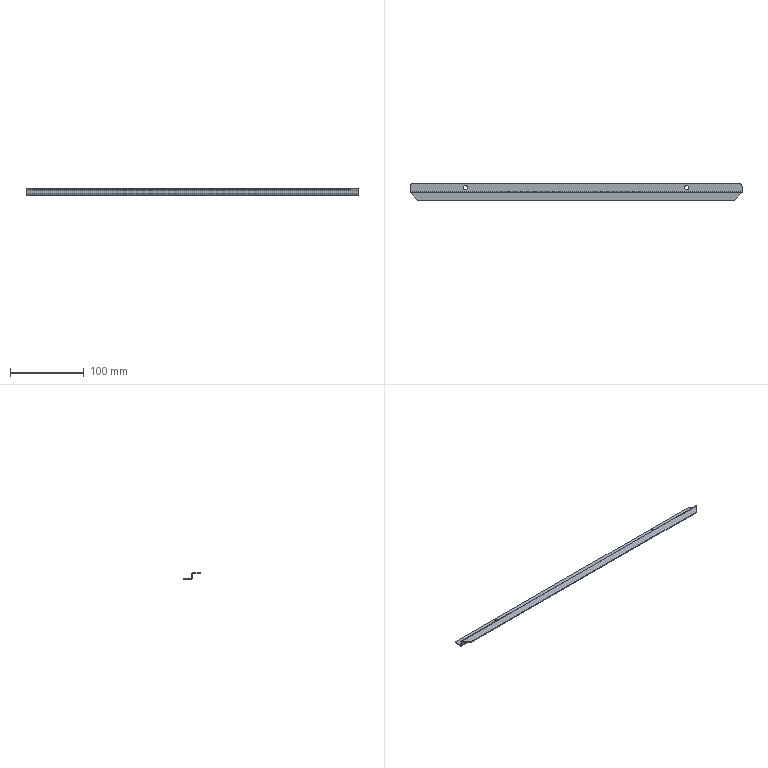Part | SolidWorks | features Chamfer 1, Fillet 1, FlatPattern 1, HoleWzd 1, SMBaseFlange 1, SheetMetal 1 | 1 solid | 28 faces | box 450 x 22 x 8.2 mm | volume 15097 mm3 | plane 18 | cylinder 10 | commonest cylinder face diameters 6 x6 0.4 x2 2.8 x2
STEP:
#1=CARTESIAN_POINT('',(-153.,7.,0.));
#2=VERTEX_POINT('',#1);
#3=CARTESIAN_POINT('',(-147.,7.,0.));
#4=VERTEX_POINT('',#3);
#5=CARTESIAN_POINT('',(-150.,7.,0.));
#6=DIRECTION('',(0.,0.,1.));
#7=DIRECTION('',(1.,0.,0.));
#8=AXIS2_PLACEMENT_3D('',#5,#6,#7);
#9=CIRCLE('',#8,3.);
#10=EDGE_CURVE('',#2,#4,#9,.T.);
#11=ORIENTED_EDGE('',*,*,#10,.F.);
#12=CARTESIAN_POINT('',(-153.,7.,1.2));
#13=VERTEX_POINT('',#12);
#14=CARTESIAN_POINT('',(-153.,7.,1.2));
#15=DIRECTION('',(0.,0.,1.));
#16=VECTOR('',#15,1000.);
#17=LINE('',#14,#16);
#18=EDGE_CURVE('',#2,#13,#17,.T.);
#19=ORIENTED_EDGE('',*,*,#18,.T.);
#20=CARTESIAN_POINT('',(-147.,7.,1.2));
#21=VERTEX_POINT('',#20);
#22=CARTESIAN_POINT('',(-150.,7.,1.2));
#23=DIRECTION('',(0.,0.,1.));
#24=DIRECTION('',(1.,0.,0.));
#25=AXIS2_PLACEMENT_3D('',#22,#23,#24);
#26=CIRCLE('',#25,3.);
#27=EDGE_CURVE('',#13,#21,#26,.T.);
#28=ORIENTED_EDGE('',*,*,#27,.T.);
#29=CARTESIAN_POINT('',(-147.,7.,1.2));
#30=DIRECTION('',(0.,0.,1.));
#31=VECTOR('',#30,1000.);
#32=LINE('',#29,#31);
#33=EDGE_CURVE('',#4,#21,#32,.T.);
#34=ORIENTED_EDGE('',*,*,#33,.F.);
#35=EDGE_LOOP('',(#11,#19,#28,#34));
#36=FACE_OUTER_BOUND('',#35,.T.);
#37=CARTESIAN_POINT('',(-150.,7.,1.2));
#38=DIRECTION('',(0.,0.,1.));
#39=DIRECTION('',(1.,0.,0.));
#40=AXIS2_PLACEMENT_3D('',#37,#38,#39);
#41=CYLINDRICAL_SURFACE('',#40,3.);
#42=ADVANCED_FACE('',(#36),#41,.F.);
#43=CARTESIAN_POINT('',(147.,7.,0.));
#44=VERTEX_POINT('',#43);
#45=CARTESIAN_POINT('',(153.,7.,0.));
#46=VERTEX_POINT('',#45);
#47=CARTESIAN_POINT('',(150.,7.,0.));
#48=DIRECTION('',(0.,0.,1.));
#49=DIRECTION('',(1.,0.,0.));
#50=AXIS2_PLACEMENT_3D('',#47,#48,#49);
#51=CIRCLE('',#50,3.);
#52=EDGE_CURVE('',#44,#46,#51,.T.);
#53=ORIENTED_EDGE('',*,*,#52,.F.);
#54=CARTESIAN_POINT('',(147.,7.,1.2));
#55=VERTEX_POINT('',#54);
#56=CARTESIAN_POINT('',(147.,7.,1.2));
#57=DIRECTION('',(0.,0.,1.));
#58=VECTOR('',#57,1000.);
#59=LINE('',#56,#58);
#60=EDGE_CURVE('',#44,#55,#59,.T.);
#61=ORIENTED_EDGE('',*,*,#60,.T.);
#62=CARTESIAN_POINT('',(153.,7.,1.2));
#63=VERTEX_POINT('',#62);
#64=CARTESIAN_POINT('',(150.,7.,1.2));
#65=DIRECTION('',(0.,0.,1.));
#66=DIRECTION('',(1.,0.,0.));
#67=AXIS2_PLACEMENT_3D('',#64,#65,#66);
#68=CIRCLE('',#67,3.);
#69=EDGE_CURVE('',#55,#63,#68,.T.);
#70=ORIENTED_EDGE('',*,*,#69,.T.);
#71=CARTESIAN_POINT('',(153.,7.,1.2));
#72=DIRECTION('',(0.,0.,1.));
#73=VECTOR('',#72,1000.);
#74=LINE('',#71,#73);
#75=EDGE_CURVE('',#46,#63,#74,.T.);
#76=ORIENTED_EDGE('',*,*,#75,.F.);
#77=EDGE_LOOP('',(#53,#61,#70,#76));
#78=FACE_OUTER_BOUND('',#77,.T.);
#79=CARTESIAN_POINT('',(150.,7.,1.2));
#80=DIRECTION('',(0.,0.,1.));
#81=DIRECTION('',(1.,0.,0.));
#82=AXIS2_PLACEMENT_3D('',#79,#80,#81);
#83=CYLINDRICAL_SURFACE('',#82,3.);
#84=ADVANCED_FACE('',(#78),#83,.F.);
#85=CARTESIAN_POINT('',(225.,0.,8.186));
#86=VERTEX_POINT('',#85);
#87=CARTESIAN_POINT('',(225.,1.2,6.8));
#88=VERTEX_POINT('',#87);
#89=CARTESIAN_POINT('',(225.,-0.2,6.8));
#90=DIRECTION('',(-1.,0.,0.));
#91=DIRECTION('',(0.,0.,-1.));
#92=AXIS2_PLACEMENT_3D('',#89,#90,#91);
#93=CIRCLE('',#92,1.4);
#94=EDGE_CURVE('',#86,#88,#93,.T.);
#95=ORIENTED_EDGE('',*,*,#94,.F.);
#96=CARTESIAN_POINT('',(225.,0.,6.8));
#97=VERTEX_POINT('',#96);
#98=CARTESIAN_POINT('',(225.,0.,7.));
#99=DIRECTION('',(0.,0.,-1.));
#100=VECTOR('',#99,1000.);
#101=LINE('',#98,#100);
#102=EDGE_CURVE('',#86,#97,#101,.T.);
#103=ORIENTED_EDGE('',*,*,#102,.T.);
#104=CARTESIAN_POINT('',(225.,1.2,6.8));
#105=DIRECTION('',(0.,-1.,0.));
#106=VECTOR('',#105,1000.);
#107=LINE('',#104,#106);
#108=EDGE_CURVE('',#88,#97,#107,.T.);
#109=ORIENTED_EDGE('',*,*,#108,.F.);
#110=EDGE_LOOP('',(#95,#103,#109));
#111=FACE_OUTER_BOUND('',#110,.T.);
#112=CARTESIAN_POINT('',(225.,-0.2,7.));
#113=DIRECTION('',(1.,0.,0.));
#114=DIRECTION('',(0.,0.,-1.));
#115=AXIS2_PLACEMENT_3D('',#112,#113,#114);
#116=PLANE('',#115);
#117=ADVANCED_FACE('',(#111),#116,.T.);
#118=CARTESIAN_POINT('',(-225.,0.,6.8));
#119=VERTEX_POINT('',#118);
#120=CARTESIAN_POINT('',(-225.,1.2,6.8));
#121=VERTEX_POINT('',#120);
#122=CARTESIAN_POINT('',(-225.,0.,6.8));
#123=DIRECTION('',(0.,1.,0.));
#124=VECTOR('',#123,1000.);
#125=LINE('',#122,#124);
#126=EDGE_CURVE('',#119,#121,#125,.T.);
#127=ORIENTED_EDGE('',*,*,#126,.F.);
#128=CARTESIAN_POINT('',(-225.,0.,8.186));
#129=VERTEX_POINT('',#128);
#130=CARTESIAN_POINT('',(-225.,0.,6.8));
#131=DIRECTION('',(0.,0.,1.));
#132=VECTOR('',#131,1000.);
#133=LINE('',#130,#132);
#134=EDGE_CURVE('',#119,#129,#133,.T.);
#135=ORIENTED_EDGE('',*,*,#134,.T.);
#136=CARTESIAN_POINT('',(-225.,-0.2,6.8));
#137=DIRECTION('',(-1.,0.,0.));
#138=DIRECTION('',(0.,0.,-1.));
#139=AXIS2_PLACEMENT_3D('',#136,#137,#138);
#140=CIRCLE('',#139,1.4);
#141=EDGE_CURVE('',#129,#121,#140,.T.);
#142=ORIENTED_EDGE('',*,*,#141,.T.);
#143=EDGE_LOOP('',(#127,#135,#142));
#144=FACE_OUTER_BOUND('',#143,.T.);
#145=CARTESIAN_POINT('',(-225.,0.,6.8));
#146=DIRECTION('',(-1.,0.,0.));
#147=DIRECTION('',(0.,0.,1.));
#148=AXIS2_PLACEMENT_3D('',#145,#146,#147);
#149=PLANE('',#148);
#150=ADVANCED_FACE('',(#144),#149,.T.);
#151=CARTESIAN_POINT('',(-225.,0.,1.4));
#152=VERTEX_POINT('',#151);
#153=CARTESIAN_POINT('',(-225.,0.,0.));
#154=DIRECTION('',(0.,0.,-1.));
#155=VECTOR('',#154,1000.);
#156=LINE('',#153,#155);
#157=EDGE_CURVE('',#119,#152,#156,.T.);
#158=ORIENTED_EDGE('',*,*,#157,.F.);
#159=ORIENTED_EDGE('',*,*,#126,.T.);
#160=CARTESIAN_POINT('',(-225.,1.2,1.4));
#161=VERTEX_POINT('',#160);
#162=CARTESIAN_POINT('',(-225.,1.2,0.));
#163=DIRECTION('',(0.,0.,-1.));
#164=VECTOR('',#163,1000.);
#165=LINE('',#162,#164);
#166=EDGE_CURVE('',#121,#161,#165,.T.);
#167=ORIENTED_EDGE('',*,*,#166,.T.);
#168=CARTESIAN_POINT('',(-225.,1.2,1.4));
#169=DIRECTION('',(0.,-1.,0.));
#170=VECTOR('',#169,1000.);
#171=LINE('',#168,#170);
#172=EDGE_CURVE('',#161,#152,#171,.T.);
#173=ORIENTED_EDGE('',*,*,#172,.T.);
#174=EDGE_LOOP('',(#158,#159,#167,#173));
#175=FACE_OUTER_BOUND('',#174,.T.);
#176=CARTESIAN_POINT('',(-225.,-0.2,8.2));
#177=DIRECTION('',(-1.,0.,0.));
#178=DIRECTION('',(0.,0.,1.));
#179=AXIS2_PLACEMENT_3D('',#176,#177,#178);
#180=PLANE('',#179);
#181=ADVANCED_FACE('',(#175),#180,.T.);
#182=CARTESIAN_POINT('',(225.,0.,1.4));
#183=VERTEX_POINT('',#182);
#184=CARTESIAN_POINT('',(225.,1.2,1.4));
#185=VERTEX_POINT('',#184);
#186=CARTESIAN_POINT('',(225.,0.,1.4));
#187=DIRECTION('',(0.,1.,0.));
#188=VECTOR('',#187,1000.);
#189=LINE('',#186,#188);
#190=EDGE_CURVE('',#183,#185,#189,.T.);
#191=ORIENTED_EDGE('',*,*,#190,.F.);
#192=CARTESIAN_POINT('',(225.,1.4,0.));
#193=VERTEX_POINT('',#192);
#194=CARTESIAN_POINT('',(225.,1.4,1.4));
#195=DIRECTION('',(1.,0.,0.));
#196=DIRECTION('',(0.,0.,1.));
#197=AXIS2_PLACEMENT_3D('',#194,#195,#196);
#198=CIRCLE('',#197,1.4);
#199=EDGE_CURVE('',#183,#193,#198,.T.);
#200=ORIENTED_EDGE('',*,*,#199,.T.);
#201=CARTESIAN_POINT('',(225.,1.4,1.2));
#202=VERTEX_POINT('',#201);
#203=CARTESIAN_POINT('',(225.,1.4,1.2));
#204=DIRECTION('',(0.,0.,-1.));
#205=VECTOR('',#204,1000.);
#206=LINE('',#203,#205);
#207=EDGE_CURVE('',#202,#193,#206,.T.);
#208=ORIENTED_EDGE('',*,*,#207,.F.);
#209=CARTESIAN_POINT('',(225.,1.4,1.4));
#210=DIRECTION('',(1.,0.,0.));
#211=DIRECTION('',(0.,0.,-1.));
#212=AXIS2_PLACEMENT_3D('',#209,#210,#211);
#213=CIRCLE('',#212,0.2);
#214=EDGE_CURVE('',#185,#202,#213,.T.);
#215=ORIENTED_EDGE('',*,*,#214,.F.);
#216=EDGE_LOOP('',(#191,#200,#208,#215));
#217=FACE_OUTER_BOUND('',#216,.T.);
#218=CARTESIAN_POINT('',(225.,0.,1.4));
#219=DIRECTION('',(1.,0.,0.));
#220=DIRECTION('',(0.,0.,-1.));
#221=AXIS2_PLACEMENT_3D('',#218,#219,#220);
#222=PLANE('',#221);
#223=ADVANCED_FACE('',(#217),#222,.T.);
#224=CARTESIAN_POINT('',(225.,0.,0.));
#225=DIRECTION('',(0.,0.,-1.));
#226=VECTOR('',#225,1000.);
#227=LINE('',#224,#226);
#228=EDGE_CURVE('',#97,#183,#227,.T.);
#229=ORIENTED_EDGE('',*,*,#228,.T.);
#230=ORIENTED_EDGE('',*,*,#190,.T.);
#231=CARTESIAN_POINT('',(225.,1.2,0.));
#232=DIRECTION('',(0.,0.,-1.));
#233=VECTOR('',#232,1000.);
#234=LINE('',#231,#233);
#235=EDGE_CURVE('',#88,#185,#234,.T.);
#236=ORIENTED_EDGE('',*,*,#235,.F.);
#237=ORIENTED_EDGE('',*,*,#108,.T.);
#238=EDGE_LOOP('',(#229,#230,#236,#237));
#239=FACE_OUTER_BOUND('',#238,.T.);
#240=CARTESIAN_POINT('',(225.,1.4,1.2));
#241=DIRECTION('',(1.,0.,0.));
#242=DIRECTION('',(0.,0.,-1.));
#243=AXIS2_PLACEMENT_3D('',#240,#241,#242);
#244=PLANE('',#243);
#245=ADVANCED_FACE('',(#239),#244,.T.);
#246=CARTESIAN_POINT('',(-225.,1.4,0.));
#247=VERTEX_POINT('',#246);
#248=CARTESIAN_POINT('',(-225.,1.4,1.2));
#249=VERTEX_POINT('',#248);
#250=CARTESIAN_POINT('',(-225.,1.4,0.));
#251=DIRECTION('',(0.,0.,1.));
#252=VECTOR('',#251,1000.);
#253=LINE('',#250,#252);
#254=EDGE_CURVE('',#247,#249,#253,.T.);
#255=ORIENTED_EDGE('',*,*,#254,.F.);
#256=CARTESIAN_POINT('',(-225.,1.4,1.4));
#257=DIRECTION('',(1.,0.,0.));
#258=DIRECTION('',(0.,0.,1.));
#259=AXIS2_PLACEMENT_3D('',#256,#257,#258);
#260=CIRCLE('',#259,1.4);
#261=EDGE_CURVE('',#152,#247,#260,.T.);
#262=ORIENTED_EDGE('',*,*,#261,.F.);
#263=ORIENTED_EDGE('',*,*,#172,.F.);
#264=CARTESIAN_POINT('',(-225.,1.4,1.4));
#265=DIRECTION('',(1.,0.,0.));
#266=DIRECTION('',(0.,0.,-1.));
#267=AXIS2_PLACEMENT_3D('',#264,#265,#266);
#268=CIRCLE('',#267,0.2);
#269=EDGE_CURVE('',#161,#249,#268,.T.);
#270=ORIENTED_EDGE('',*,*,#269,.T.);
#271=EDGE_LOOP('',(#255,#262,#263,#270));
#272=FACE_OUTER_BOUND('',#271,.T.);
#273=CARTESIAN_POINT('',(-225.,1.4,0.));
#274=DIRECTION('',(-1.,0.,0.));
#275=DIRECTION('',(0.,0.,1.));
#276=AXIS2_PLACEMENT_3D('',#273,#274,#275);
#277=PLANE('',#276);
#278=ADVANCED_FACE('',(#272),#277,.T.);
#279=CARTESIAN_POINT('',(-225.,9.,1.2));
#280=VERTEX_POINT('',#279);
#281=CARTESIAN_POINT('',(-225.,0.,1.2));
#282=DIRECTION('',(0.,1.,0.));
#283=VECTOR('',#282,1000.);
#284=LINE('',#281,#283);
#285=EDGE_CURVE('',#249,#280,#284,.T.);
#286=ORIENTED_EDGE('',*,*,#285,.T.);
#287=CARTESIAN_POINT('',(-225.,9.,0.));
#288=VERTEX_POINT('',#287);
#289=CARTESIAN_POINT('',(-225.,9.,1.4));
#290=DIRECTION('',(0.,0.,-1.));
#291=VECTOR('',#290,1000.);
#292=LINE('',#289,#291);
#293=EDGE_CURVE('',#280,#288,#292,.T.);
#294=ORIENTED_EDGE('',*,*,#293,.T.);
#295=CARTESIAN_POINT('',(-225.,0.,0.));
#296=DIRECTION('',(0.,1.,0.));
#297=VECTOR('',#296,1000.);
#298=LINE('',#295,#297);
#299=EDGE_CURVE('',#247,#288,#298,.T.);
#300=ORIENTED_EDGE('',*,*,#299,.F.);
#301=ORIENTED_EDGE('',*,*,#254,.T.);
#302=EDGE_LOOP('',(#286,#294,#300,#301));
#303=FACE_OUTER_BOUND('',#302,.T.);
#304=CARTESIAN_POINT('',(-225.,1.2,1.4));
#305=DIRECTION('',(-1.,0.,0.));
#306=DIRECTION('',(0.,0.,1.));
#307=AXIS2_PLACEMENT_3D('',#304,#305,#306);
#308=PLANE('',#307);
#309=ADVANCED_FACE('',(#303),#308,.T.);
#310=CARTESIAN_POINT('',(-150.,7.,0.));
#311=DIRECTION('',(0.,0.,1.));
#312=DIRECTION('',(1.,0.,0.));
#313=AXIS2_PLACEMENT_3D('',#310,#311,#312);
#314=CIRCLE('',#313,3.);
#315=EDGE_CURVE('',#4,#2,#314,.T.);
#316=ORIENTED_EDGE('',*,*,#315,.T.);
#317=ORIENTED_EDGE('',*,*,#10,.T.);
#318=EDGE_LOOP('',(#316,#317));
#319=FACE_BOUND('',#318,.T.);
#320=CARTESIAN_POINT('',(150.,7.,0.));
#321=DIRECTION('',(0.,0.,1.));
#322=DIRECTION('',(1.,0.,0.));
#323=AXIS2_PLACEMENT_3D('',#320,#321,#322);
#324=CIRCLE('',#323,3.);
#325=EDGE_CURVE('',#46,#44,#324,.T.);
#326=ORIENTED_EDGE('',*,*,#325,.T.);
#327=ORIENTED_EDGE('',*,*,#52,.T.);
#328=EDGE_LOOP('',(#326,#327));
#329=FACE_BOUND('',#328,.T.);
#330=ORIENTED_EDGE('',*,*,#299,.T.);
#331=CARTESIAN_POINT('',(-222.,12.,0.));
#332=VERTEX_POINT('',#331);
#333=CARTESIAN_POINT('',(-222.,9.,0.));
#334=DIRECTION('',(0.,0.,-1.));
#335=DIRECTION('',(1.,0.,0.));
#336=AXIS2_PLACEMENT_3D('',#333,#334,#335);
#337=CIRCLE('',#336,3.);
#338=EDGE_CURVE('',#288,#332,#337,.T.);
#339=ORIENTED_EDGE('',*,*,#338,.T.);
#340=CARTESIAN_POINT('',(222.,12.,0.));
#341=VERTEX_POINT('',#340);
#342=CARTESIAN_POINT('',(225.,12.,0.));
#343=DIRECTION('',(-1.,0.,0.));
#344=VECTOR('',#343,1000.);
#345=LINE('',#342,#344);
#346=EDGE_CURVE('',#341,#332,#345,.T.);
#347=ORIENTED_EDGE('',*,*,#346,.F.);
#348=CARTESIAN_POINT('',(225.,9.,0.));
#349=VERTEX_POINT('',#348);
#350=CARTESIAN_POINT('',(222.,9.,0.));
#351=DIRECTION('',(0.,0.,-1.));
#352=DIRECTION('',(1.,0.,0.));
#353=AXIS2_PLACEMENT_3D('',#350,#351,#352);
#354=CIRCLE('',#353,3.);
#355=EDGE_CURVE('',#341,#349,#354,.T.);
#356=ORIENTED_EDGE('',*,*,#355,.T.);
#357=CARTESIAN_POINT('',(225.,0.,0.));
#358=DIRECTION('',(0.,1.,0.));
#359=VECTOR('',#358,1000.);
#360=LINE('',#357,#359);
#361=EDGE_CURVE('',#193,#349,#360,.T.);
#362=ORIENTED_EDGE('',*,*,#361,.F.);
#363=CARTESIAN_POINT('',(225.,1.4,0.));
#364=DIRECTION('',(-1.,0.,0.));
#365=VECTOR('',#364,1000.);
#366=LINE('',#363,#365);
#367=EDGE_CURVE('',#193,#247,#366,.T.);
#368=ORIENTED_EDGE('',*,*,#367,.T.);
#369=EDGE_LOOP('',(#330,#339,#347,#356,#362,#368));
#370=FACE_OUTER_BOUND('',#369,.T.);
#371=CARTESIAN_POINT('',(225.,0.,0.));
#372=DIRECTION('',(0.,0.,1.));
#373=DIRECTION('',(1.,0.,0.));
#374=AXIS2_PLACEMENT_3D('',#371,#372,#373);
#375=PLANE('',#374);
#376=ADVANCED_FACE('',(#319,#329,#370),#375,.F.);
#377=ORIENTED_EDGE('',*,*,#346,.T.);
#378=CARTESIAN_POINT('',(-222.,12.,1.2));
#379=VERTEX_POINT('',#378);
#380=CARTESIAN_POINT('',(-222.,12.,1.2));
#381=DIRECTION('',(0.,0.,1.));
#382=VECTOR('',#381,1000.);
#383=LINE('',#380,#382);
#384=EDGE_CURVE('',#332,#379,#383,.T.);
#385=ORIENTED_EDGE('',*,*,#384,.T.);
#386=CARTESIAN_POINT('',(222.,12.,1.2));
#387=VERTEX_POINT('',#386);
#388=CARTESIAN_POINT('',(225.,12.,1.2));
#389=DIRECTION('',(-1.,0.,0.));
#390=VECTOR('',#389,1000.);
#391=LINE('',#388,#390);
#392=EDGE_CURVE('',#387,#379,#391,.T.);
#393=ORIENTED_EDGE('',*,*,#392,.F.);
#394=CARTESIAN_POINT('',(222.,12.,1.2));
#395=DIRECTION('',(0.,0.,-1.));
#396=VECTOR('',#395,1000.);
#397=LINE('',#394,#396);
#398=EDGE_CURVE('',#387,#341,#397,.T.);
#399=ORIENTED_EDGE('',*,*,#398,.T.);
#400=EDGE_LOOP('',(#377,#385,#393,#399));
#401=FACE_OUTER_BOUND('',#400,.T.);
#402=CARTESIAN_POINT('',(225.,12.,1.2));
#403=DIRECTION('',(0.,1.,0.));
#404=DIRECTION('',(0.,0.,1.));
#405=AXIS2_PLACEMENT_3D('',#402,#403,#404);
#406=PLANE('',#405);
#407=ADVANCED_FACE('',(#401),#406,.T.);
#408=CARTESIAN_POINT('',(-150.,7.,1.2));
#409=DIRECTION('',(0.,0.,1.));
#410=DIRECTION('',(1.,0.,0.));
#411=AXIS2_PLACEMENT_3D('',#408,#409,#410);
#412=CIRCLE('',#411,3.);
#413=EDGE_CURVE('',#21,#13,#412,.T.);
#414=ORIENTED_EDGE('',*,*,#413,.F.);
#415=ORIENTED_EDGE('',*,*,#27,.F.);
#416=EDGE_LOOP('',(#414,#415));
#417=FACE_BOUND('',#416,.T.);
#418=CARTESIAN_POINT('',(150.,7.,1.2));
#419=DIRECTION('',(0.,0.,1.));
#420=DIRECTION('',(1.,0.,0.));
#421=AXIS2_PLACEMENT_3D('',#418,#419,#420);
#422=CIRCLE('',#421,3.);
#423=EDGE_CURVE('',#63,#55,#422,.T.);
#424=ORIENTED_EDGE('',*,*,#423,.F.);
#425=ORIENTED_EDGE('',*,*,#69,.F.);
#426=EDGE_LOOP('',(#424,#425));
#427=FACE_BOUND('',#426,.T.);
#428=ORIENTED_EDGE('',*,*,#392,.T.);
#429=CARTESIAN_POINT('',(-222.,9.,1.2));
#430=DIRECTION('',(0.,0.,1.));
#431=DIRECTION('',(1.,0.,0.));
#432=AXIS2_PLACEMENT_3D('',#429,#430,#431);
#433=CIRCLE('',#432,3.);
#434=EDGE_CURVE('',#379,#280,#433,.T.);
#435=ORIENTED_EDGE('',*,*,#434,.T.);
#436=ORIENTED_EDGE('',*,*,#285,.F.);
#437=CARTESIAN_POINT('',(225.,1.4,1.2));
#438=DIRECTION('',(-1.,0.,0.));
#439=VECTOR('',#438,1000.);
#440=LINE('',#437,#439);
#441=EDGE_CURVE('',#202,#249,#440,.T.);
#442=ORIENTED_EDGE('',*,*,#441,.F.);
#443=CARTESIAN_POINT('',(225.,9.,1.2));
#444=VERTEX_POINT('',#443);
#445=CARTESIAN_POINT('',(225.,0.,1.2));
#446=DIRECTION('',(0.,1.,0.));
#447=VECTOR('',#446,1000.);
#448=LINE('',#445,#447);
#449=EDGE_CURVE('',#202,#444,#448,.T.);
#450=ORIENTED_EDGE('',*,*,#449,.T.);
#451=CARTESIAN_POINT('',(222.,9.,1.2));
#452=DIRECTION('',(0.,0.,1.));
#453=DIRECTION('',(1.,0.,0.));
#454=AXIS2_PLACEMENT_3D('',#451,#452,#453);
#455=CIRCLE('',#454,3.);
#456=EDGE_CURVE('',#444,#387,#455,.T.);
#457=ORIENTED_EDGE('',*,*,#456,.T.);
#458=EDGE_LOOP('',(#428,#435,#436,#442,#450,#457));
#459=FACE_OUTER_BOUND('',#458,.T.);
#460=CARTESIAN_POINT('',(225.,0.,1.2));
#461=DIRECTION('',(0.,0.,1.));
#462=DIRECTION('',(1.,0.,0.));
#463=AXIS2_PLACEMENT_3D('',#460,#461,#462);
#464=PLANE('',#463);
#465=ADVANCED_FACE('',(#417,#427,#459),#464,.T.);
#466=ORIENTED_EDGE('',*,*,#269,.F.);
#467=CARTESIAN_POINT('',(225.,1.2,1.4));
#468=DIRECTION('',(-1.,0.,0.));
#469=VECTOR('',#468,1000.);
#470=LINE('',#467,#469);
#471=EDGE_CURVE('',#185,#161,#470,.T.);
#472=ORIENTED_EDGE('',*,*,#471,.F.);
#473=ORIENTED_EDGE('',*,*,#214,.T.);
#474=ORIENTED_EDGE('',*,*,#441,.T.);
#475=EDGE_LOOP('',(#466,#472,#473,#474));
#476=FACE_OUTER_BOUND('',#475,.T.);
#477=CARTESIAN_POINT('',(225.,1.4,1.4));
#478=DIRECTION('',(-1.,0.,0.));
#479=DIRECTION('',(0.,0.,1.));
#480=AXIS2_PLACEMENT_3D('',#477,#478,#479);
#481=CYLINDRICAL_SURFACE('',#480,0.2);
#482=ADVANCED_FACE('',(#476),#481,.F.);
#483=ORIENTED_EDGE('',*,*,#166,.F.);
#484=CARTESIAN_POINT('',(225.,1.2,6.8));
#485=DIRECTION('',(-1.,0.,0.));
#486=VECTOR('',#485,1000.);
#487=LINE('',#484,#486);
#488=EDGE_CURVE('',#88,#121,#487,.T.);
#489=ORIENTED_EDGE('',*,*,#488,.F.);
#490=ORIENTED_EDGE('',*,*,#235,.T.);
#491=ORIENTED_EDGE('',*,*,#471,.T.);
#492=EDGE_LOOP('',(#483,#489,#490,#491));
#493=FACE_OUTER_BOUND('',#492,.T.);
#494=CARTESIAN_POINT('',(225.,1.2,0.));
#495=DIRECTION('',(0.,1.,0.));
#496=DIRECTION('',(0.,0.,1.));
#497=AXIS2_PLACEMENT_3D('',#494,#495,#496);
#498=PLANE('',#497);
#499=ADVANCED_FACE('',(#493),#498,.T.);
#500=CARTESIAN_POINT('',(224.8,-0.2,8.2));
#501=VERTEX_POINT('',#500);
#502=CARTESIAN_POINT('',(-224.8,-0.2,8.2));
#503=VERTEX_POINT('',#502);
#504=CARTESIAN_POINT('',(225.,-0.2,8.2));
#505=DIRECTION('',(-1.,0.,0.));
#506=VECTOR('',#505,1000.);
#507=LINE('',#504,#506);
#508=EDGE_CURVE('',#501,#503,#507,.T.);
#509=ORIENTED_EDGE('',*,*,#508,.F.);
#510=CARTESIAN_POINT('',(224.8,-0.2,8.2));
#511=CARTESIAN_POINT('',(224.867,-0.133,8.2));
#512=CARTESIAN_POINT('',(224.934,-0.06627,8.195));
#513=CARTESIAN_POINT('',(225.,0.,8.186));
#514=(BOUNDED_CURVE()B_SPLINE_CURVE(3,(#510,#511,#512,#513),.UNSPECIFIED.,.F.,.T.)B_SPLINE_CURVE_WITH_KNOTS((4,4),(1.571,1.714),.UNSPECIFIED.)CURVE()GEOMETRIC_REPRESENTATION_ITEM()RATIONAL_B_SPLINE_CURVE((1.,0.9983,0.9983,1.))REPRESENTATION_ITEM(''));
#515=EDGE_CURVE('',#501,#86,#514,.T.);
#516=ORIENTED_EDGE('',*,*,#515,.T.);
#517=ORIENTED_EDGE('',*,*,#94,.T.);
#518=ORIENTED_EDGE('',*,*,#488,.T.);
#519=ORIENTED_EDGE('',*,*,#141,.F.);
#520=CARTESIAN_POINT('',(-225.,0.,8.186));
#521=CARTESIAN_POINT('',(-224.934,-0.06627,8.195));
#522=CARTESIAN_POINT('',(-224.867,-0.133,8.2));
#523=CARTESIAN_POINT('',(-224.8,-0.2,8.2));
#524=(BOUNDED_CURVE()B_SPLINE_CURVE(3,(#520,#521,#522,#523),.UNSPECIFIED.,.F.,.T.)B_SPLINE_CURVE_WITH_KNOTS((4,4),(1.427,1.571),.UNSPECIFIED.)CURVE()GEOMETRIC_REPRESENTATION_ITEM()RATIONAL_B_SPLINE_CURVE((1.,0.9983,0.9983,1.))REPRESENTATION_ITEM(''));
#525=EDGE_CURVE('',#129,#503,#524,.T.);
#526=ORIENTED_EDGE('',*,*,#525,.T.);
#527=EDGE_LOOP('',(#509,#516,#517,#518,#519,#526));
#528=FACE_OUTER_BOUND('',#527,.T.);
#529=CARTESIAN_POINT('',(225.,-0.2,6.8));
#530=DIRECTION('',(-1.,0.,0.));
#531=DIRECTION('',(0.,0.,1.));
#532=AXIS2_PLACEMENT_3D('',#529,#530,#531);
#533=CYLINDRICAL_SURFACE('',#532,1.4);
#534=ADVANCED_FACE('',(#528),#533,.T.);
#535=CARTESIAN_POINT('',(215.,-10.,8.2));
#536=VERTEX_POINT('',#535);
#537=CARTESIAN_POINT('',(-215.,-10.,8.2));
#538=VERTEX_POINT('',#537);
#539=CARTESIAN_POINT('',(225.,-10.,8.2));
#540=DIRECTION('',(-1.,0.,0.));
#541=VECTOR('',#540,1000.);
#542=LINE('',#539,#541);
#543=EDGE_CURVE('',#536,#538,#542,.T.);
#544=ORIENTED_EDGE('',*,*,#543,.F.);
#545=CARTESIAN_POINT('',(225.,0.,8.2));
#546=DIRECTION('',(0.7071,0.7071,0.));
#547=VECTOR('',#546,1000.);
#548=LINE('',#545,#547);
#549=EDGE_CURVE('',#536,#501,#548,.T.);
#550=ORIENTED_EDGE('',*,*,#549,.T.);
#551=ORIENTED_EDGE('',*,*,#508,.T.);
#552=CARTESIAN_POINT('',(0.,-225.,8.2));
#553=DIRECTION('',(0.7071,-0.7071,0.));
#554=VECTOR('',#553,1000.);
#555=LINE('',#552,#554);
#556=EDGE_CURVE('',#503,#538,#555,.T.);
#557=ORIENTED_EDGE('',*,*,#556,.T.);
#558=EDGE_LOOP('',(#544,#550,#551,#557));
#559=FACE_OUTER_BOUND('',#558,.T.);
#560=CARTESIAN_POINT('',(225.,0.,8.2));
#561=DIRECTION('',(0.,0.,1.));
#562=DIRECTION('',(0.,-1.,0.));
#563=AXIS2_PLACEMENT_3D('',#560,#561,#562);
#564=PLANE('',#563);
#565=ADVANCED_FACE('',(#559),#564,.T.);
#566=CARTESIAN_POINT('',(215.,-10.,7.));
#567=VERTEX_POINT('',#566);
#568=CARTESIAN_POINT('',(-215.,-10.,7.));
#569=VERTEX_POINT('',#568);
#570=CARTESIAN_POINT('',(225.,-10.,7.));
#571=DIRECTION('',(-1.,0.,0.));
#572=VECTOR('',#571,1000.);
#573=LINE('',#570,#572);
#574=EDGE_CURVE('',#567,#569,#573,.T.);
#575=ORIENTED_EDGE('',*,*,#574,.F.);
#576=CARTESIAN_POINT('',(215.,-10.,7.));
#577=DIRECTION('',(0.,0.,1.));
#578=VECTOR('',#577,1000.);
#579=LINE('',#576,#578);
#580=EDGE_CURVE('',#567,#536,#579,.T.);
#581=ORIENTED_EDGE('',*,*,#580,.T.);
#582=ORIENTED_EDGE('',*,*,#543,.T.);
#583=CARTESIAN_POINT('',(-215.,-10.,7.));
#584=DIRECTION('',(0.,0.,-1.));
#585=VECTOR('',#584,1000.);
#586=LINE('',#583,#585);
#587=EDGE_CURVE('',#538,#569,#586,.T.);
#588=ORIENTED_EDGE('',*,*,#587,.T.);
#589=EDGE_LOOP('',(#575,#581,#582,#588));
#590=FACE_OUTER_BOUND('',#589,.T.);
#591=CARTESIAN_POINT('',(225.,-10.,7.));
#592=DIRECTION('',(0.,-1.,0.));
#593=DIRECTION('',(0.,0.,-1.));
#594=AXIS2_PLACEMENT_3D('',#591,#592,#593);
#595=PLANE('',#594);
#596=ADVANCED_FACE('',(#590),#595,.T.);
#597=CARTESIAN_POINT('',(224.8,-0.2,7.));
#598=VERTEX_POINT('',#597);
#599=CARTESIAN_POINT('',(-224.8,-0.2,7.));
#600=VERTEX_POINT('',#599);
#601=CARTESIAN_POINT('',(225.,-0.2,7.));
#602=DIRECTION('',(-1.,0.,0.));
#603=VECTOR('',#602,1000.);
#604=LINE('',#601,#603);
#605=EDGE_CURVE('',#598,#600,#604,.T.);
#606=ORIENTED_EDGE('',*,*,#605,.F.);
#607=CARTESIAN_POINT('',(215.,-10.,7.));
#608=DIRECTION('',(-0.7071,-0.7071,0.));
#609=VECTOR('',#608,1000.);
#610=LINE('',#607,#609);
#611=EDGE_CURVE('',#598,#567,#610,.T.);
#612=ORIENTED_EDGE('',*,*,#611,.T.);
#613=ORIENTED_EDGE('',*,*,#574,.T.);
#614=CARTESIAN_POINT('',(-225.,0.,7.));
#615=DIRECTION('',(-0.7071,0.7071,0.));
#616=VECTOR('',#615,1000.);
#617=LINE('',#614,#616);
#618=EDGE_CURVE('',#569,#600,#617,.T.);
#619=ORIENTED_EDGE('',*,*,#618,.T.);
#620=EDGE_LOOP('',(#606,#612,#613,#619));
#621=FACE_OUTER_BOUND('',#620,.T.);
#622=CARTESIAN_POINT('',(225.,0.,7.));
#623=DIRECTION('',(0.,0.,1.));
#624=DIRECTION('',(0.,-1.,0.));
#625=AXIS2_PLACEMENT_3D('',#622,#623,#624);
#626=PLANE('',#625);
#627=ADVANCED_FACE('',(#621),#626,.F.);
#628=CARTESIAN_POINT('',(225.,0.,6.8));
#629=DIRECTION('',(-1.,0.,0.));
#630=VECTOR('',#629,1000.);
#631=LINE('',#628,#630);
#632=EDGE_CURVE('',#97,#119,#631,.T.);
#633=ORIENTED_EDGE('',*,*,#632,.F.);
#634=CARTESIAN_POINT('',(225.,0.,6.8));
#635=CARTESIAN_POINT('',(225.,0.,6.917));
#636=CARTESIAN_POINT('',(224.917,-0.08284,7.));
#637=CARTESIAN_POINT('',(224.8,-0.2,7.));
#638=(BOUNDED_CURVE()B_SPLINE_CURVE(3,(#634,#635,#636,#637),.UNSPECIFIED.,.F.,.F.)B_SPLINE_CURVE_WITH_KNOTS((4,4),(3.142,4.712),.UNSPECIFIED.)CURVE()GEOMETRIC_REPRESENTATION_ITEM()RATIONAL_B_SPLINE_CURVE((1.,0.8047,0.8047,1.))REPRESENTATION_ITEM(''));
#639=EDGE_CURVE('',#97,#598,#638,.T.);
#640=ORIENTED_EDGE('',*,*,#639,.T.);
#641=ORIENTED_EDGE('',*,*,#605,.T.);
#642=CARTESIAN_POINT('',(-224.8,-0.2,7.));
#643=CARTESIAN_POINT('',(-224.917,-0.08284,7.));
#644=CARTESIAN_POINT('',(-225.,0.,6.917));
#645=CARTESIAN_POINT('',(-225.,0.,6.8));
#646=(BOUNDED_CURVE()B_SPLINE_CURVE(3,(#642,#643,#644,#645),.UNSPECIFIED.,.F.,.T.)B_SPLINE_CURVE_WITH_KNOTS((4,4),(4.712,6.283),.UNSPECIFIED.)CURVE()GEOMETRIC_REPRESENTATION_ITEM()RATIONAL_B_SPLINE_CURVE((1.,0.8047,0.8047,1.))REPRESENTATION_ITEM(''));
#647=EDGE_CURVE('',#600,#119,#646,.T.);
#648=ORIENTED_EDGE('',*,*,#647,.T.);
#649=EDGE_LOOP('',(#633,#640,#641,#648));
#650=FACE_OUTER_BOUND('',#649,.T.);
#651=CARTESIAN_POINT('',(225.,-0.2,6.8));
#652=DIRECTION('',(-1.,0.,0.));
#653=DIRECTION('',(0.,0.,1.));
#654=AXIS2_PLACEMENT_3D('',#651,#652,#653);
#655=CYLINDRICAL_SURFACE('',#654,0.2);
#656=ADVANCED_FACE('',(#650),#655,.F.);
#657=ORIENTED_EDGE('',*,*,#157,.T.);
#658=CARTESIAN_POINT('',(225.,0.,1.4));
#659=DIRECTION('',(-1.,0.,0.));
#660=VECTOR('',#659,1000.);
#661=LINE('',#658,#660);
#662=EDGE_CURVE('',#183,#152,#661,.T.);
#663=ORIENTED_EDGE('',*,*,#662,.F.);
#664=ORIENTED_EDGE('',*,*,#228,.F.);
#665=ORIENTED_EDGE('',*,*,#632,.T.);
#666=EDGE_LOOP('',(#657,#663,#664,#665));
#667=FACE_OUTER_BOUND('',#666,.T.);
#668=CARTESIAN_POINT('',(225.,0.,0.));
#669=DIRECTION('',(0.,1.,0.));
#670=DIRECTION('',(0.,0.,1.));
#671=AXIS2_PLACEMENT_3D('',#668,#669,#670);
#672=PLANE('',#671);
#673=ADVANCED_FACE('',(#667),#672,.F.);
#674=ORIENTED_EDGE('',*,*,#261,.T.);
#675=ORIENTED_EDGE('',*,*,#367,.F.);
#676=ORIENTED_EDGE('',*,*,#199,.F.);
#677=ORIENTED_EDGE('',*,*,#662,.T.);
#678=EDGE_LOOP('',(#674,#675,#676,#677));
#679=FACE_OUTER_BOUND('',#678,.T.);
#680=CARTESIAN_POINT('',(225.,1.4,1.4));
#681=DIRECTION('',(-1.,0.,0.));
#682=DIRECTION('',(0.,0.,1.));
#683=AXIS2_PLACEMENT_3D('',#680,#681,#682);
#684=CYLINDRICAL_SURFACE('',#683,1.4);
#685=ADVANCED_FACE('',(#679),#684,.T.);
#686=ORIENTED_EDGE('',*,*,#361,.T.);
#687=CARTESIAN_POINT('',(225.,9.,1.4));
#688=DIRECTION('',(0.,0.,1.));
#689=VECTOR('',#688,1000.);
#690=LINE('',#687,#689);
#691=EDGE_CURVE('',#349,#444,#690,.T.);
#692=ORIENTED_EDGE('',*,*,#691,.T.);
#693=ORIENTED_EDGE('',*,*,#449,.F.);
#694=ORIENTED_EDGE('',*,*,#207,.T.);
#695=EDGE_LOOP('',(#686,#692,#693,#694));
#696=FACE_OUTER_BOUND('',#695,.T.);
#697=CARTESIAN_POINT('',(225.,1.4,1.4));
#698=DIRECTION('',(1.,0.,0.));
#699=DIRECTION('',(0.,0.,-1.));
#700=AXIS2_PLACEMENT_3D('',#697,#698,#699);
#701=PLANE('',#700);
#702=ADVANCED_FACE('',(#696),#701,.T.);
#703=ORIENTED_EDGE('',*,*,#60,.F.);
#704=ORIENTED_EDGE('',*,*,#325,.F.);
#705=ORIENTED_EDGE('',*,*,#75,.T.);
#706=ORIENTED_EDGE('',*,*,#423,.T.);
#707=EDGE_LOOP('',(#703,#704,#705,#706));
#708=FACE_OUTER_BOUND('',#707,.T.);
#709=CARTESIAN_POINT('',(150.,7.,1.2));
#710=DIRECTION('',(0.,0.,1.));
#711=DIRECTION('',(1.,0.,0.));
#712=AXIS2_PLACEMENT_3D('',#709,#710,#711);
#713=CYLINDRICAL_SURFACE('',#712,3.);
#714=ADVANCED_FACE('',(#708),#713,.F.);
#715=ORIENTED_EDGE('',*,*,#18,.F.);
#716=ORIENTED_EDGE('',*,*,#315,.F.);
#717=ORIENTED_EDGE('',*,*,#33,.T.);
#718=ORIENTED_EDGE('',*,*,#413,.T.);
#719=EDGE_LOOP('',(#715,#716,#717,#718));
#720=FACE_OUTER_BOUND('',#719,.T.);
#721=CARTESIAN_POINT('',(-150.,7.,1.2));
#722=DIRECTION('',(0.,0.,1.));
#723=DIRECTION('',(1.,0.,0.));
#724=AXIS2_PLACEMENT_3D('',#721,#722,#723);
#725=CYLINDRICAL_SURFACE('',#724,3.);
#726=ADVANCED_FACE('',(#720),#725,.F.);
#727=ORIENTED_EDGE('',*,*,#639,.F.);
#728=ORIENTED_EDGE('',*,*,#102,.F.);
#729=ORIENTED_EDGE('',*,*,#515,.F.);
#730=ORIENTED_EDGE('',*,*,#549,.F.);
#731=ORIENTED_EDGE('',*,*,#580,.F.);
#732=ORIENTED_EDGE('',*,*,#611,.F.);
#733=EDGE_LOOP('',(#727,#728,#729,#730,#731,#732));
#734=FACE_OUTER_BOUND('',#733,.T.);
#735=CARTESIAN_POINT('',(215.,-10.,7.));
#736=DIRECTION('',(-0.7071,0.7071,0.));
#737=DIRECTION('',(0.,0.,1.));
#738=AXIS2_PLACEMENT_3D('',#735,#736,#737);
#739=PLANE('',#738);
#740=ADVANCED_FACE('',(#734),#739,.F.);
#741=ORIENTED_EDGE('',*,*,#618,.F.);
#742=ORIENTED_EDGE('',*,*,#587,.F.);
#743=ORIENTED_EDGE('',*,*,#556,.F.);
#744=ORIENTED_EDGE('',*,*,#525,.F.);
#745=ORIENTED_EDGE('',*,*,#134,.F.);
#746=ORIENTED_EDGE('',*,*,#647,.F.);
#747=EDGE_LOOP('',(#741,#742,#743,#744,#745,#746));
#748=FACE_OUTER_BOUND('',#747,.T.);
#749=CARTESIAN_POINT('',(-225.,0.,6.8));
#750=DIRECTION('',(0.7071,0.7071,0.));
#751=DIRECTION('',(0.,0.,1.));
#752=AXIS2_PLACEMENT_3D('',#749,#750,#751);
#753=PLANE('',#752);
#754=ADVANCED_FACE('',(#748),#753,.F.);
#755=ORIENTED_EDGE('',*,*,#434,.F.);
#756=ORIENTED_EDGE('',*,*,#384,.F.);
#757=ORIENTED_EDGE('',*,*,#338,.F.);
#758=ORIENTED_EDGE('',*,*,#293,.F.);
#759=EDGE_LOOP('',(#755,#756,#757,#758));
#760=FACE_OUTER_BOUND('',#759,.T.);
#761=CARTESIAN_POINT('',(-222.,9.,1.4));
#762=DIRECTION('',(0.,0.,-1.));
#763=DIRECTION('',(-1.,0.,0.));
#764=AXIS2_PLACEMENT_3D('',#761,#762,#763);
#765=CYLINDRICAL_SURFACE('',#764,3.);
#766=ADVANCED_FACE('',(#760),#765,.T.);
#767=ORIENTED_EDGE('',*,*,#456,.F.);
#768=ORIENTED_EDGE('',*,*,#691,.F.);
#769=ORIENTED_EDGE('',*,*,#355,.F.);
#770=ORIENTED_EDGE('',*,*,#398,.F.);
#771=EDGE_LOOP('',(#767,#768,#769,#770));
#772=FACE_OUTER_BOUND('',#771,.T.);
#773=CARTESIAN_POINT('',(222.,9.,1.2));
#774=DIRECTION('',(0.,0.,-1.));
#775=DIRECTION('',(-1.,0.,0.));
#776=AXIS2_PLACEMENT_3D('',#773,#774,#775);
#777=CYLINDRICAL_SURFACE('',#776,3.);
#778=ADVANCED_FACE('',(#772),#777,.T.);
#779=CLOSED_SHELL('',(#42,#84,#117,#150,#181,#223,#245,#278,#309,#376,#407,#465,#482,#499,#534,#565,#596,#627,#656,#673,#685,#702,#714,#726,#740,#754,#766,#778));
#780=MANIFOLD_SOLID_BREP('',#779);
#781=CARTESIAN_POINT('',(0.,0.,0.));
#782=DIRECTION('',(0.,0.,1.));
#783=DIRECTION('',(1.,0.,0.));
#784=AXIS2_PLACEMENT_3D('',#781,#782,#783);
#785=(LENGTH_UNIT()NAMED_UNIT(*)SI_UNIT(.MILLI.,.METRE.));
#786=UNCERTAINTY_MEASURE_WITH_UNIT(LENGTH_MEASURE(0.00001),#785,'','');
#787=(NAMED_UNIT(*)PLANE_ANGLE_UNIT()SI_UNIT($,.RADIAN.));
#788=(NAMED_UNIT(*)SI_UNIT($,.STERADIAN.)SOLID_ANGLE_UNIT());
#789=(GEOMETRIC_REPRESENTATION_CONTEXT(3)GLOBAL_UNCERTAINTY_ASSIGNED_CONTEXT((#786))GLOBAL_UNIT_ASSIGNED_CONTEXT((#785,#787,#788))REPRESENTATION_CONTEXT('',''));
#790=ADVANCED_BREP_SHAPE_REPRESENTATION('',(#780,#784),#789);